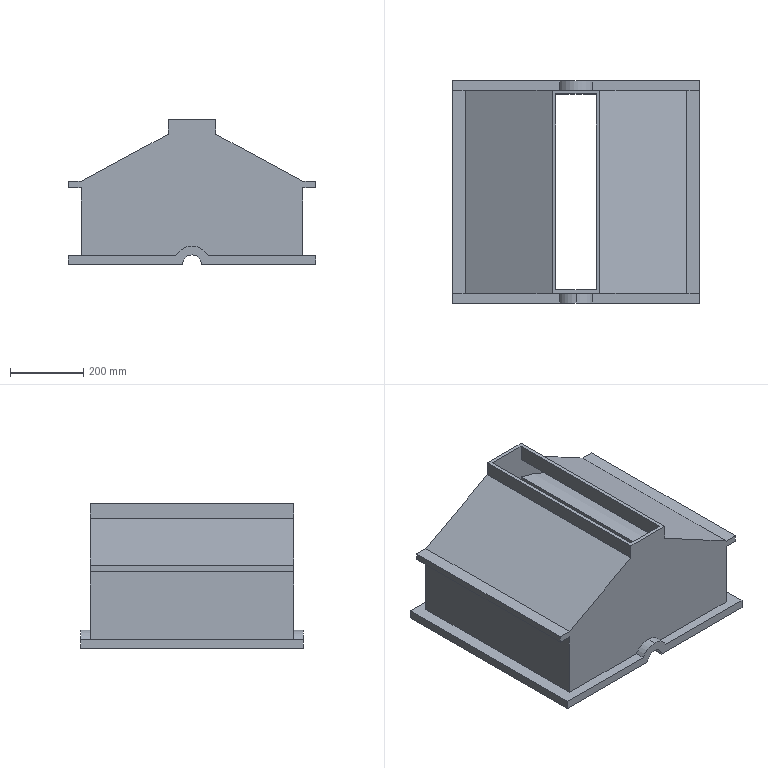Part | SolidWorks | features ICE 5, MirrorPattern 4, Extrusion 1 | 1 solid | 44 faces | box 677.491 x 608 x 396.469 mm | volume 20641288 mm3 | plane 33 | cylinder 11 | commonest cylinder face diameters 52 x4 100 x3 556 x2 596 x2
STEP:
#1=CARTESIAN_POINT('',(5.246,268.,26.));
#2=VERTEX_POINT('',#1);
#3=CARTESIAN_POINT('',(31.246,268.,0.));
#4=VERTEX_POINT('',#3);
#5=CARTESIAN_POINT('',(5.246,268.,0.));
#6=DIRECTION('',(0.,1.,0.));
#7=DIRECTION('',(0.,0.,1.));
#8=AXIS2_PLACEMENT_3D('',#5,#6,#7);
#9=CIRCLE('',#8,26.);
#10=EDGE_CURVE('',#2,#4,#9,.T.);
#11=ORIENTED_EDGE('',*,*,#10,.F.);
#12=CARTESIAN_POINT('',(5.246,304.,26.));
#13=VERTEX_POINT('',#12);
#14=CARTESIAN_POINT('',(5.246,-304.,26.));
#15=DIRECTION('',(0.,1.,0.));
#16=VECTOR('',#15,1000.);
#17=LINE('',#14,#16);
#18=EDGE_CURVE('',#2,#13,#17,.T.);
#19=ORIENTED_EDGE('',*,*,#18,.T.);
#20=CARTESIAN_POINT('',(31.246,304.,0.));
#21=VERTEX_POINT('',#20);
#22=CARTESIAN_POINT('',(5.246,304.,0.));
#23=DIRECTION('',(0.,1.,0.));
#24=DIRECTION('',(0.,0.,1.));
#25=AXIS2_PLACEMENT_3D('',#22,#23,#24);
#26=CIRCLE('',#25,26.);
#27=EDGE_CURVE('',#13,#21,#26,.T.);
#28=ORIENTED_EDGE('',*,*,#27,.T.);
#29=CARTESIAN_POINT('',(31.246,-304.,0.));
#30=DIRECTION('',(0.,1.,0.));
#31=VECTOR('',#30,1000.);
#32=LINE('',#29,#31);
#33=EDGE_CURVE('',#4,#21,#32,.T.);
#34=ORIENTED_EDGE('',*,*,#33,.F.);
#35=EDGE_LOOP('',(#11,#19,#28,#34));
#36=FACE_OUTER_BOUND('',#35,.T.);
#37=CARTESIAN_POINT('',(5.246,-304.,0.));
#38=DIRECTION('',(0.,1.,0.));
#39=DIRECTION('',(0.,0.,1.));
#40=AXIS2_PLACEMENT_3D('',#37,#38,#39);
#41=CYLINDRICAL_SURFACE('',#40,26.);
#42=ADVANCED_FACE('',(#36),#41,.F.);
#43=CARTESIAN_POINT('',(31.246,-304.,0.));
#44=VERTEX_POINT('',#43);
#45=CARTESIAN_POINT('',(5.246,-304.,26.));
#46=VERTEX_POINT('',#45);
#47=CARTESIAN_POINT('',(5.246,-304.,0.));
#48=DIRECTION('',(0.,-1.,0.));
#49=DIRECTION('',(0.,0.,-1.));
#50=AXIS2_PLACEMENT_3D('',#47,#48,#49);
#51=CIRCLE('',#50,26.);
#52=EDGE_CURVE('',#44,#46,#51,.T.);
#53=ORIENTED_EDGE('',*,*,#52,.T.);
#54=CARTESIAN_POINT('',(5.246,-268.,26.));
#55=VERTEX_POINT('',#54);
#56=CARTESIAN_POINT('',(5.246,-304.,26.));
#57=DIRECTION('',(0.,1.,0.));
#58=VECTOR('',#57,1000.);
#59=LINE('',#56,#58);
#60=EDGE_CURVE('',#46,#55,#59,.T.);
#61=ORIENTED_EDGE('',*,*,#60,.T.);
#62=CARTESIAN_POINT('',(31.246,-268.,0.));
#63=VERTEX_POINT('',#62);
#64=CARTESIAN_POINT('',(5.246,-268.,0.));
#65=DIRECTION('',(0.,-1.,0.));
#66=DIRECTION('',(0.,0.,-1.));
#67=AXIS2_PLACEMENT_3D('',#64,#65,#66);
#68=CIRCLE('',#67,26.);
#69=EDGE_CURVE('',#63,#55,#68,.T.);
#70=ORIENTED_EDGE('',*,*,#69,.F.);
#71=CARTESIAN_POINT('',(31.246,-304.,0.));
#72=DIRECTION('',(0.,1.,0.));
#73=VECTOR('',#72,1000.);
#74=LINE('',#71,#73);
#75=EDGE_CURVE('',#44,#63,#74,.T.);
#76=ORIENTED_EDGE('',*,*,#75,.F.);
#77=EDGE_LOOP('',(#53,#61,#70,#76));
#78=FACE_OUTER_BOUND('',#77,.T.);
#79=CARTESIAN_POINT('',(5.246,-304.,0.));
#80=DIRECTION('',(0.,1.,0.));
#81=DIRECTION('',(0.,0.,1.));
#82=AXIS2_PLACEMENT_3D('',#79,#80,#81);
#83=CYLINDRICAL_SURFACE('',#82,26.);
#84=ADVANCED_FACE('',(#78),#83,.F.);
#85=CARTESIAN_POINT('',(-38.618,-304.,24.));
#86=VERTEX_POINT('',#85);
#87=CARTESIAN_POINT('',(5.246,-304.,50.));
#88=VERTEX_POINT('',#87);
#89=CARTESIAN_POINT('',(5.246,-304.,0.));
#90=DIRECTION('',(0.,1.,0.));
#91=DIRECTION('',(0.,0.,1.));
#92=AXIS2_PLACEMENT_3D('',#89,#90,#91);
#93=CIRCLE('',#92,50.);
#94=EDGE_CURVE('',#86,#88,#93,.T.);
#95=ORIENTED_EDGE('',*,*,#94,.T.);
#96=CARTESIAN_POINT('',(5.246,-278.,50.));
#97=VERTEX_POINT('',#96);
#98=CARTESIAN_POINT('',(5.246,-304.,50.));
#99=DIRECTION('',(0.,1.,0.));
#100=VECTOR('',#99,1000.);
#101=LINE('',#98,#100);
#102=EDGE_CURVE('',#88,#97,#101,.T.);
#103=ORIENTED_EDGE('',*,*,#102,.T.);
#104=CARTESIAN_POINT('',(-38.618,-278.,24.));
#105=VERTEX_POINT('',#104);
#106=CARTESIAN_POINT('',(5.246,-278.,0.));
#107=DIRECTION('',(0.,1.,0.));
#108=DIRECTION('',(0.,0.,1.));
#109=AXIS2_PLACEMENT_3D('',#106,#107,#108);
#110=CIRCLE('',#109,50.);
#111=EDGE_CURVE('',#105,#97,#110,.T.);
#112=ORIENTED_EDGE('',*,*,#111,.F.);
#113=CARTESIAN_POINT('',(-38.618,-304.,24.));
#114=DIRECTION('',(0.,1.,0.));
#115=VECTOR('',#114,1000.);
#116=LINE('',#113,#115);
#117=EDGE_CURVE('',#86,#105,#116,.T.);
#118=ORIENTED_EDGE('',*,*,#117,.F.);
#119=EDGE_LOOP('',(#95,#103,#112,#118));
#120=FACE_OUTER_BOUND('',#119,.T.);
#121=CARTESIAN_POINT('',(5.246,-304.,0.));
#122=DIRECTION('',(0.,1.,0.));
#123=DIRECTION('',(0.,0.,1.));
#124=AXIS2_PLACEMENT_3D('',#121,#122,#123);
#125=CYLINDRICAL_SURFACE('',#124,50.);
#126=ADVANCED_FACE('',(#120),#125,.T.);
#127=CARTESIAN_POINT('',(343.991,-304.,0.));
#128=VERTEX_POINT('',#127);
#129=CARTESIAN_POINT('',(-333.5,-304.,0.));
#130=DIRECTION('',(1.,0.,0.));
#131=VECTOR('',#130,1000.);
#132=LINE('',#129,#131);
#133=EDGE_CURVE('',#44,#128,#132,.T.);
#134=ORIENTED_EDGE('',*,*,#133,.F.);
#135=ORIENTED_EDGE('',*,*,#75,.T.);
#136=CARTESIAN_POINT('',(288.491,-268.,0.));
#137=VERTEX_POINT('',#136);
#138=CARTESIAN_POINT('',(-298.,-268.,0.));
#139=DIRECTION('',(-1.,0.,0.));
#140=VECTOR('',#139,1000.);
#141=LINE('',#138,#140);
#142=EDGE_CURVE('',#137,#63,#141,.T.);
#143=ORIENTED_EDGE('',*,*,#142,.F.);
#144=CARTESIAN_POINT('',(288.491,268.,0.));
#145=VERTEX_POINT('',#144);
#146=CARTESIAN_POINT('',(288.491,278.,0.));
#147=DIRECTION('',(0.,-1.,0.));
#148=VECTOR('',#147,1000.);
#149=LINE('',#146,#148);
#150=EDGE_CURVE('',#145,#137,#149,.T.);
#151=ORIENTED_EDGE('',*,*,#150,.F.);
#152=CARTESIAN_POINT('',(-298.,268.,0.));
#153=DIRECTION('',(-1.,0.,0.));
#154=VECTOR('',#153,1000.);
#155=LINE('',#152,#154);
#156=EDGE_CURVE('',#145,#4,#155,.T.);
#157=ORIENTED_EDGE('',*,*,#156,.T.);
#158=ORIENTED_EDGE('',*,*,#33,.T.);
#159=CARTESIAN_POINT('',(343.991,304.,0.));
#160=VERTEX_POINT('',#159);
#161=CARTESIAN_POINT('',(-333.5,304.,0.));
#162=DIRECTION('',(1.,0.,0.));
#163=VECTOR('',#162,1000.);
#164=LINE('',#161,#163);
#165=EDGE_CURVE('',#21,#160,#164,.T.);
#166=ORIENTED_EDGE('',*,*,#165,.T.);
#167=CARTESIAN_POINT('',(343.991,278.,0.));
#168=DIRECTION('',(0.,-1.,0.));
#169=VECTOR('',#168,1000.);
#170=LINE('',#167,#169);
#171=EDGE_CURVE('',#160,#128,#170,.T.);
#172=ORIENTED_EDGE('',*,*,#171,.T.);
#173=EDGE_LOOP('',(#134,#135,#143,#151,#157,#158,#166,#172));
#174=FACE_OUTER_BOUND('',#173,.T.);
#175=CARTESIAN_POINT('',(0.,278.,0.));
#176=DIRECTION('',(0.,0.,1.));
#177=DIRECTION('',(1.,0.,0.));
#178=AXIS2_PLACEMENT_3D('',#175,#176,#177);
#179=PLANE('',#178);
#180=ADVANCED_FACE('',(#174),#179,.F.);
#181=CARTESIAN_POINT('',(308.491,-278.,24.));
#182=VERTEX_POINT('',#181);
#183=CARTESIAN_POINT('',(49.109,-278.,24.));
#184=VERTEX_POINT('',#183);
#185=CARTESIAN_POINT('',(343.991,-278.,24.));
#186=DIRECTION('',(-1.,0.,0.));
#187=VECTOR('',#186,1000.);
#188=LINE('',#185,#187);
#189=EDGE_CURVE('',#182,#184,#188,.T.);
#190=ORIENTED_EDGE('',*,*,#189,.F.);
#191=CARTESIAN_POINT('',(308.491,-278.,209.58));
#192=VERTEX_POINT('',#191);
#193=CARTESIAN_POINT('',(308.491,-278.,209.359));
#194=DIRECTION('',(0.,0.,1.));
#195=VECTOR('',#194,1000.);
#196=LINE('',#193,#195);
#197=EDGE_CURVE('',#182,#192,#196,.T.);
#198=ORIENTED_EDGE('',*,*,#197,.T.);
#199=CARTESIAN_POINT('',(343.991,-278.,209.58));
#200=VERTEX_POINT('',#199);
#201=CARTESIAN_POINT('',(10.491,-278.,209.58));
#202=DIRECTION('',(1.,0.,0.));
#203=VECTOR('',#202,1000.);
#204=LINE('',#201,#203);
#205=EDGE_CURVE('',#192,#200,#204,.T.);
#206=ORIENTED_EDGE('',*,*,#205,.T.);
#207=CARTESIAN_POINT('',(343.991,-278.,228.));
#208=VERTEX_POINT('',#207);
#209=CARTESIAN_POINT('',(343.991,-278.,0.));
#210=DIRECTION('',(0.,0.,1.));
#211=VECTOR('',#210,1000.);
#212=LINE('',#209,#211);
#213=EDGE_CURVE('',#200,#208,#212,.T.);
#214=ORIENTED_EDGE('',*,*,#213,.T.);
#215=CARTESIAN_POINT('',(308.491,-278.,228.));
#216=VERTEX_POINT('',#215);
#217=CARTESIAN_POINT('',(10.491,-278.,228.));
#218=DIRECTION('',(-1.,0.,0.));
#219=VECTOR('',#218,1000.);
#220=LINE('',#217,#219);
#221=EDGE_CURVE('',#208,#216,#220,.T.);
#222=ORIENTED_EDGE('',*,*,#221,.T.);
#223=CARTESIAN_POINT('',(70.491,-278.,356.469));
#224=VERTEX_POINT('',#223);
#225=CARTESIAN_POINT('',(308.491,-278.,228.));
#226=DIRECTION('',(-0.88,0.,0.475));
#227=VECTOR('',#226,1000.);
#228=LINE('',#225,#227);
#229=EDGE_CURVE('',#216,#224,#228,.T.);
#230=ORIENTED_EDGE('',*,*,#229,.T.);
#231=CARTESIAN_POINT('',(70.491,-278.,396.469));
#232=VERTEX_POINT('',#231);
#233=CARTESIAN_POINT('',(70.491,-278.,356.469));
#234=DIRECTION('',(0.,0.,1.));
#235=VECTOR('',#234,1000.);
#236=LINE('',#233,#235);
#237=EDGE_CURVE('',#224,#232,#236,.T.);
#238=ORIENTED_EDGE('',*,*,#237,.T.);
#239=CARTESIAN_POINT('',(-60.,-278.,396.469));
#240=VERTEX_POINT('',#239);
#241=CARTESIAN_POINT('',(0.,-278.,396.469));
#242=DIRECTION('',(-1.,0.,0.));
#243=VECTOR('',#242,1000.);
#244=LINE('',#241,#243);
#245=EDGE_CURVE('',#232,#240,#244,.T.);
#246=ORIENTED_EDGE('',*,*,#245,.T.);
#247=CARTESIAN_POINT('',(-60.,-278.,356.469));
#248=VERTEX_POINT('',#247);
#249=CARTESIAN_POINT('',(-60.,-278.,0.));
#250=DIRECTION('',(0.,0.,-1.));
#251=VECTOR('',#250,1000.);
#252=LINE('',#249,#251);
#253=EDGE_CURVE('',#240,#248,#252,.T.);
#254=ORIENTED_EDGE('',*,*,#253,.T.);
#255=CARTESIAN_POINT('',(-298.,-278.,228.));
#256=VERTEX_POINT('',#255);
#257=CARTESIAN_POINT('',(-162.54,-278.,301.119));
#258=DIRECTION('',(-0.88,0.,-0.475));
#259=VECTOR('',#258,1000.);
#260=LINE('',#257,#259);
#261=EDGE_CURVE('',#248,#256,#260,.T.);
#262=ORIENTED_EDGE('',*,*,#261,.T.);
#263=CARTESIAN_POINT('',(-333.5,-278.,228.));
#264=VERTEX_POINT('',#263);
#265=CARTESIAN_POINT('',(0.,-278.,228.));
#266=DIRECTION('',(1.,0.,0.));
#267=VECTOR('',#266,1000.);
#268=LINE('',#265,#267);
#269=EDGE_CURVE('',#264,#256,#268,.T.);
#270=ORIENTED_EDGE('',*,*,#269,.F.);
#271=CARTESIAN_POINT('',(-333.5,-278.,209.58));
#272=VERTEX_POINT('',#271);
#273=CARTESIAN_POINT('',(-333.5,-278.,0.));
#274=DIRECTION('',(0.,0.,1.));
#275=VECTOR('',#274,1000.);
#276=LINE('',#273,#275);
#277=EDGE_CURVE('',#272,#264,#276,.T.);
#278=ORIENTED_EDGE('',*,*,#277,.F.);
#279=CARTESIAN_POINT('',(-298.,-278.,209.58));
#280=VERTEX_POINT('',#279);
#281=CARTESIAN_POINT('',(0.,-278.,209.58));
#282=DIRECTION('',(-1.,0.,0.));
#283=VECTOR('',#282,1000.);
#284=LINE('',#281,#283);
#285=EDGE_CURVE('',#280,#272,#284,.T.);
#286=ORIENTED_EDGE('',*,*,#285,.F.);
#287=CARTESIAN_POINT('',(-298.,-278.,24.));
#288=VERTEX_POINT('',#287);
#289=CARTESIAN_POINT('',(-298.,-278.,0.));
#290=DIRECTION('',(0.,0.,1.));
#291=VECTOR('',#290,1000.);
#292=LINE('',#289,#291);
#293=EDGE_CURVE('',#288,#280,#292,.T.);
#294=ORIENTED_EDGE('',*,*,#293,.F.);
#295=CARTESIAN_POINT('',(-333.5,-278.,24.));
#296=DIRECTION('',(1.,0.,0.));
#297=VECTOR('',#296,1000.);
#298=LINE('',#295,#297);
#299=EDGE_CURVE('',#288,#105,#298,.T.);
#300=ORIENTED_EDGE('',*,*,#299,.T.);
#301=ORIENTED_EDGE('',*,*,#111,.T.);
#302=CARTESIAN_POINT('',(5.246,-278.,0.));
#303=DIRECTION('',(0.,1.,0.));
#304=DIRECTION('',(0.,0.,1.));
#305=AXIS2_PLACEMENT_3D('',#302,#303,#304);
#306=CIRCLE('',#305,50.);
#307=EDGE_CURVE('',#97,#184,#306,.T.);
#308=ORIENTED_EDGE('',*,*,#307,.T.);
#309=EDGE_LOOP('',(#190,#198,#206,#214,#222,#230,#238,#246,#254,#262,#270,#278,#286,#294,#300,#301,#308));
#310=FACE_OUTER_BOUND('',#309,.T.);
#311=CARTESIAN_POINT('',(0.,-278.,0.));
#312=DIRECTION('',(0.,1.,0.));
#313=DIRECTION('',(0.,0.,1.));
#314=AXIS2_PLACEMENT_3D('',#311,#312,#313);
#315=PLANE('',#314);
#316=ADVANCED_FACE('',(#310),#315,.F.);
#317=CARTESIAN_POINT('',(49.109,278.,24.));
#318=VERTEX_POINT('',#317);
#319=CARTESIAN_POINT('',(308.491,278.,24.));
#320=VERTEX_POINT('',#319);
#321=CARTESIAN_POINT('',(343.991,278.,24.));
#322=DIRECTION('',(1.,0.,0.));
#323=VECTOR('',#322,1000.);
#324=LINE('',#321,#323);
#325=EDGE_CURVE('',#318,#320,#324,.T.);
#326=ORIENTED_EDGE('',*,*,#325,.F.);
#327=CARTESIAN_POINT('',(-38.618,278.,24.));
#328=VERTEX_POINT('',#327);
#329=CARTESIAN_POINT('',(5.246,278.,0.));
#330=DIRECTION('',(0.,1.,0.));
#331=DIRECTION('',(0.,0.,1.));
#332=AXIS2_PLACEMENT_3D('',#329,#330,#331);
#333=CIRCLE('',#332,50.);
#334=EDGE_CURVE('',#328,#318,#333,.T.);
#335=ORIENTED_EDGE('',*,*,#334,.F.);
#336=CARTESIAN_POINT('',(-298.,278.,24.));
#337=VERTEX_POINT('',#336);
#338=CARTESIAN_POINT('',(-333.5,278.,24.));
#339=DIRECTION('',(1.,0.,0.));
#340=VECTOR('',#339,1000.);
#341=LINE('',#338,#340);
#342=EDGE_CURVE('',#337,#328,#341,.T.);
#343=ORIENTED_EDGE('',*,*,#342,.F.);
#344=CARTESIAN_POINT('',(-298.,278.,209.58));
#345=VERTEX_POINT('',#344);
#346=CARTESIAN_POINT('',(-298.,278.,0.));
#347=DIRECTION('',(0.,0.,1.));
#348=VECTOR('',#347,1000.);
#349=LINE('',#346,#348);
#350=EDGE_CURVE('',#337,#345,#349,.T.);
#351=ORIENTED_EDGE('',*,*,#350,.T.);
#352=CARTESIAN_POINT('',(-333.5,278.,209.58));
#353=VERTEX_POINT('',#352);
#354=CARTESIAN_POINT('',(0.,278.,209.58));
#355=DIRECTION('',(-1.,0.,0.));
#356=VECTOR('',#355,1000.);
#357=LINE('',#354,#356);
#358=EDGE_CURVE('',#345,#353,#357,.T.);
#359=ORIENTED_EDGE('',*,*,#358,.T.);
#360=CARTESIAN_POINT('',(-333.5,278.,228.));
#361=VERTEX_POINT('',#360);
#362=CARTESIAN_POINT('',(-333.5,278.,0.));
#363=DIRECTION('',(0.,0.,1.));
#364=VECTOR('',#363,1000.);
#365=LINE('',#362,#364);
#366=EDGE_CURVE('',#353,#361,#365,.T.);
#367=ORIENTED_EDGE('',*,*,#366,.T.);
#368=CARTESIAN_POINT('',(-298.,278.,228.));
#369=VERTEX_POINT('',#368);
#370=CARTESIAN_POINT('',(0.,278.,228.));
#371=DIRECTION('',(1.,0.,0.));
#372=VECTOR('',#371,1000.);
#373=LINE('',#370,#372);
#374=EDGE_CURVE('',#361,#369,#373,.T.);
#375=ORIENTED_EDGE('',*,*,#374,.T.);
#376=CARTESIAN_POINT('',(-60.,278.,356.469));
#377=VERTEX_POINT('',#376);
#378=CARTESIAN_POINT('',(-162.54,278.,301.119));
#379=DIRECTION('',(-0.88,0.,-0.475));
#380=VECTOR('',#379,1000.);
#381=LINE('',#378,#380);
#382=EDGE_CURVE('',#377,#369,#381,.T.);
#383=ORIENTED_EDGE('',*,*,#382,.F.);
#384=CARTESIAN_POINT('',(-60.,278.,396.469));
#385=VERTEX_POINT('',#384);
#386=CARTESIAN_POINT('',(-60.,278.,0.));
#387=DIRECTION('',(0.,0.,-1.));
#388=VECTOR('',#387,1000.);
#389=LINE('',#386,#388);
#390=EDGE_CURVE('',#385,#377,#389,.T.);
#391=ORIENTED_EDGE('',*,*,#390,.F.);
#392=CARTESIAN_POINT('',(70.491,278.,396.469));
#393=VERTEX_POINT('',#392);
#394=CARTESIAN_POINT('',(0.,278.,396.469));
#395=DIRECTION('',(-1.,0.,0.));
#396=VECTOR('',#395,1000.);
#397=LINE('',#394,#396);
#398=EDGE_CURVE('',#393,#385,#397,.T.);
#399=ORIENTED_EDGE('',*,*,#398,.F.);
#400=CARTESIAN_POINT('',(70.491,278.,356.469));
#401=VERTEX_POINT('',#400);
#402=CARTESIAN_POINT('',(70.491,278.,356.469));
#403=DIRECTION('',(0.,0.,1.));
#404=VECTOR('',#403,1000.);
#405=LINE('',#402,#404);
#406=EDGE_CURVE('',#401,#393,#405,.T.);
#407=ORIENTED_EDGE('',*,*,#406,.F.);
#408=CARTESIAN_POINT('',(308.491,278.,228.));
#409=VERTEX_POINT('',#408);
#410=CARTESIAN_POINT('',(308.491,278.,228.));
#411=DIRECTION('',(-0.88,0.,0.475));
#412=VECTOR('',#411,1000.);
#413=LINE('',#410,#412);
#414=EDGE_CURVE('',#409,#401,#413,.T.);
#415=ORIENTED_EDGE('',*,*,#414,.F.);
#416=CARTESIAN_POINT('',(343.991,278.,228.));
#417=VERTEX_POINT('',#416);
#418=CARTESIAN_POINT('',(10.491,278.,228.));
#419=DIRECTION('',(-1.,0.,0.));
#420=VECTOR('',#419,1000.);
#421=LINE('',#418,#420);
#422=EDGE_CURVE('',#417,#409,#421,.T.);
#423=ORIENTED_EDGE('',*,*,#422,.F.);
#424=CARTESIAN_POINT('',(343.991,278.,209.58));
#425=VERTEX_POINT('',#424);
#426=CARTESIAN_POINT('',(343.991,278.,0.));
#427=DIRECTION('',(0.,0.,1.));
#428=VECTOR('',#427,1000.);
#429=LINE('',#426,#428);
#430=EDGE_CURVE('',#425,#417,#429,.T.);
#431=ORIENTED_EDGE('',*,*,#430,.F.);
#432=CARTESIAN_POINT('',(308.491,278.,209.58));
#433=VERTEX_POINT('',#432);
#434=CARTESIAN_POINT('',(10.491,278.,209.58));
#435=DIRECTION('',(1.,0.,0.));
#436=VECTOR('',#435,1000.);
#437=LINE('',#434,#436);
#438=EDGE_CURVE('',#433,#425,#437,.T.);
#439=ORIENTED_EDGE('',*,*,#438,.F.);
#440=CARTESIAN_POINT('',(308.491,278.,209.359));
#441=DIRECTION('',(0.,0.,1.));
#442=VECTOR('',#441,1000.);
#443=LINE('',#440,#442);
#444=EDGE_CURVE('',#320,#433,#443,.T.);
#445=ORIENTED_EDGE('',*,*,#444,.F.);
#446=EDGE_LOOP('',(#326,#335,#343,#351,#359,#367,#375,#383,#391,#399,#407,#415,#423,#431,#439,#445));
#447=FACE_OUTER_BOUND('',#446,.T.);
#448=CARTESIAN_POINT('',(0.,278.,0.));
#449=DIRECTION('',(0.,1.,0.));
#450=DIRECTION('',(0.,0.,1.));
#451=AXIS2_PLACEMENT_3D('',#448,#449,#450);
#452=PLANE('',#451);
#453=ADVANCED_FACE('',(#447),#452,.T.);
#454=CARTESIAN_POINT('',(-286.793,-268.,80.955));
#455=VERTEX_POINT('',#454);
#456=CARTESIAN_POINT('',(-285.175,-268.,220.714));
#457=VERTEX_POINT('',#456);
#458=CARTESIAN_POINT('',(-287.692,-268.,3.331));
#459=DIRECTION('',(0.01158,0.,0.9999));
#460=VECTOR('',#459,1000.);
#461=LINE('',#458,#460);
#462=EDGE_CURVE('',#455,#457,#461,.T.);
#463=ORIENTED_EDGE('',*,*,#462,.F.);
#464=CARTESIAN_POINT('',(-286.793,268.,80.955));
#465=VERTEX_POINT('',#464);
#466=CARTESIAN_POINT('',(-286.793,278.,80.955));
#467=DIRECTION('',(0.,-1.,0.));
#468=VECTOR('',#467,1000.);
#469=LINE('',#466,#468);
#470=EDGE_CURVE('',#465,#455,#469,.T.);
#471=ORIENTED_EDGE('',*,*,#470,.F.);
#472=CARTESIAN_POINT('',(-285.175,268.,220.714));
#473=VERTEX_POINT('',#472);
#474=CARTESIAN_POINT('',(-287.692,268.,3.331));
#475=DIRECTION('',(-0.01158,0.,-0.9999));
#476=VECTOR('',#475,1000.);
#477=LINE('',#474,#476);
#478=EDGE_CURVE('',#473,#465,#477,.T.);
#479=ORIENTED_EDGE('',*,*,#478,.F.);
#480=CARTESIAN_POINT('',(-285.175,278.,220.714));
#481=DIRECTION('',(0.,-1.,0.));
#482=VECTOR('',#481,1000.);
#483=LINE('',#480,#482);
#484=EDGE_CURVE('',#473,#457,#483,.T.);
#485=ORIENTED_EDGE('',*,*,#484,.T.);
#486=EDGE_LOOP('',(#463,#471,#479,#485));
#487=FACE_OUTER_BOUND('',#486,.T.);
#488=CARTESIAN_POINT('',(-287.692,278.,3.331));
#489=DIRECTION('',(-0.9999,0.,0.01158));
#490=DIRECTION('',(0.01158,0.,0.9999));
#491=AXIS2_PLACEMENT_3D('',#488,#489,#490);
#492=PLANE('',#491);
#493=ADVANCED_FACE('',(#487),#492,.F.);
#494=CARTESIAN_POINT('',(-49.909,-268.,293.791));
#495=VERTEX_POINT('',#494);
#496=CARTESIAN_POINT('',(0.,-268.,0.));
#497=DIRECTION('',(0.,-1.,0.));
#498=DIRECTION('',(0.,0.,-1.));
#499=AXIS2_PLACEMENT_3D('',#496,#497,#498);
#500=CIRCLE('',#499,298.);
#501=EDGE_CURVE('',#495,#455,#500,.T.);
#502=ORIENTED_EDGE('',*,*,#501,.F.);
#503=CARTESIAN_POINT('',(-49.909,268.,293.791));
#504=VERTEX_POINT('',#503);
#505=CARTESIAN_POINT('',(-49.909,278.,293.791));
#506=DIRECTION('',(0.,-1.,0.));
#507=VECTOR('',#506,1000.);
#508=LINE('',#505,#507);
#509=EDGE_CURVE('',#504,#495,#508,.T.);
#510=ORIENTED_EDGE('',*,*,#509,.F.);
#511=CARTESIAN_POINT('',(0.,268.,0.));
#512=DIRECTION('',(0.,1.,0.));
#513=DIRECTION('',(0.,0.,1.));
#514=AXIS2_PLACEMENT_3D('',#511,#512,#513);
#515=CIRCLE('',#514,298.);
#516=EDGE_CURVE('',#465,#504,#515,.T.);
#517=ORIENTED_EDGE('',*,*,#516,.F.);
#518=ORIENTED_EDGE('',*,*,#470,.T.);
#519=EDGE_LOOP('',(#502,#510,#517,#518));
#520=FACE_OUTER_BOUND('',#519,.T.);
#521=CARTESIAN_POINT('',(0.,278.,0.));
#522=DIRECTION('',(0.,-1.,0.));
#523=DIRECTION('',(0.,0.,-1.));
#524=AXIS2_PLACEMENT_3D('',#521,#522,#523);
#525=CYLINDRICAL_SURFACE('',#524,298.);
#526=ADVANCED_FACE('',(#520),#525,.T.);
#527=ORIENTED_EDGE('',*,*,#509,.T.);
#528=CARTESIAN_POINT('',(-49.909,-268.,273.483));
#529=VERTEX_POINT('',#528);
#530=CARTESIAN_POINT('',(-49.909,-268.,0.));
#531=DIRECTION('',(0.,0.,-1.));
#532=VECTOR('',#531,1000.);
#533=LINE('',#530,#532);
#534=EDGE_CURVE('',#495,#529,#533,.T.);
#535=ORIENTED_EDGE('',*,*,#534,.T.);
#536=CARTESIAN_POINT('',(-49.909,268.,273.483));
#537=VERTEX_POINT('',#536);
#538=CARTESIAN_POINT('',(-49.909,278.,273.483));
#539=DIRECTION('',(0.,-1.,0.));
#540=VECTOR('',#539,1000.);
#541=LINE('',#538,#540);
#542=EDGE_CURVE('',#537,#529,#541,.T.);
#543=ORIENTED_EDGE('',*,*,#542,.F.);
#544=CARTESIAN_POINT('',(-49.909,268.,0.));
#545=DIRECTION('',(0.,0.,1.));
#546=VECTOR('',#545,1000.);
#547=LINE('',#544,#546);
#548=EDGE_CURVE('',#537,#504,#547,.T.);
#549=ORIENTED_EDGE('',*,*,#548,.T.);
#550=EDGE_LOOP('',(#527,#535,#543,#549));
#551=FACE_OUTER_BOUND('',#550,.T.);
#552=CARTESIAN_POINT('',(-49.909,278.,0.));
#553=DIRECTION('',(1.,0.,0.));
#554=DIRECTION('',(0.,0.,-1.));
#555=AXIS2_PLACEMENT_3D('',#552,#553,#554);
#556=PLANE('',#555);
#557=ADVANCED_FACE('',(#551),#556,.T.);
#558=ORIENTED_EDGE('',*,*,#542,.T.);
#559=CARTESIAN_POINT('',(-278.,-268.,0.));
#560=VERTEX_POINT('',#559);
#561=CARTESIAN_POINT('',(0.,-268.,0.));
#562=DIRECTION('',(0.,-1.,0.));
#563=DIRECTION('',(0.,0.,-1.));
#564=AXIS2_PLACEMENT_3D('',#561,#562,#563);
#565=CIRCLE('',#564,278.);
#566=EDGE_CURVE('',#529,#560,#565,.T.);
#567=ORIENTED_EDGE('',*,*,#566,.T.);
#568=CARTESIAN_POINT('',(-278.,268.,0.));
#569=VERTEX_POINT('',#568);
#570=CARTESIAN_POINT('',(-278.,278.,0.));
#571=DIRECTION('',(0.,-1.,0.));
#572=VECTOR('',#571,1000.);
#573=LINE('',#570,#572);
#574=EDGE_CURVE('',#569,#560,#573,.T.);
#575=ORIENTED_EDGE('',*,*,#574,.F.);
#576=CARTESIAN_POINT('',(0.,268.,0.));
#577=DIRECTION('',(0.,1.,0.));
#578=DIRECTION('',(0.,0.,1.));
#579=AXIS2_PLACEMENT_3D('',#576,#577,#578);
#580=CIRCLE('',#579,278.);
#581=EDGE_CURVE('',#569,#537,#580,.T.);
#582=ORIENTED_EDGE('',*,*,#581,.T.);
#583=EDGE_LOOP('',(#558,#567,#575,#582));
#584=FACE_OUTER_BOUND('',#583,.T.);
#585=CARTESIAN_POINT('',(0.,278.,0.));
#586=DIRECTION('',(0.,-1.,0.));
#587=DIRECTION('',(0.,0.,-1.));
#588=AXIS2_PLACEMENT_3D('',#585,#586,#587);
#589=CYLINDRICAL_SURFACE('',#588,278.);
#590=ADVANCED_FACE('',(#584),#589,.F.);
#591=CARTESIAN_POINT('',(-49.909,-268.,352.336));
#592=VERTEX_POINT('',#591);
#593=CARTESIAN_POINT('',(-49.909,-268.,396.469));
#594=VERTEX_POINT('',#593);
#595=CARTESIAN_POINT('',(-49.909,-268.,0.));
#596=DIRECTION('',(0.,0.,1.));
#597=VECTOR('',#596,1000.);
#598=LINE('',#595,#597);
#599=EDGE_CURVE('',#592,#594,#598,.T.);
#600=ORIENTED_EDGE('',*,*,#599,.F.);
#601=CARTESIAN_POINT('',(-49.909,268.,352.336));
#602=VERTEX_POINT('',#601);
#603=CARTESIAN_POINT('',(-49.909,278.,352.336));
#604=DIRECTION('',(0.,-1.,0.));
#605=VECTOR('',#604,1000.);
#606=LINE('',#603,#605);
#607=EDGE_CURVE('',#602,#592,#606,.T.);
#608=ORIENTED_EDGE('',*,*,#607,.F.);
#609=CARTESIAN_POINT('',(-49.909,268.,396.469));
#610=VERTEX_POINT('',#609);
#611=CARTESIAN_POINT('',(-49.909,268.,0.));
#612=DIRECTION('',(0.,0.,-1.));
#613=VECTOR('',#612,1000.);
#614=LINE('',#611,#613);
#615=EDGE_CURVE('',#610,#602,#614,.T.);
#616=ORIENTED_EDGE('',*,*,#615,.F.);
#617=CARTESIAN_POINT('',(-49.909,278.,396.469));
#618=DIRECTION('',(0.,-1.,0.));
#619=VECTOR('',#618,1000.);
#620=LINE('',#617,#619);
#621=EDGE_CURVE('',#610,#594,#620,.T.);
#622=ORIENTED_EDGE('',*,*,#621,.T.);
#623=EDGE_LOOP('',(#600,#608,#616,#622));
#624=FACE_OUTER_BOUND('',#623,.T.);
#625=CARTESIAN_POINT('',(-49.909,278.,0.));
#626=DIRECTION('',(-1.,0.,0.));
#627=DIRECTION('',(0.,0.,1.));
#628=AXIS2_PLACEMENT_3D('',#625,#626,#627);
#629=PLANE('',#628);
#630=ADVANCED_FACE('',(#624),#629,.F.);
#631=CARTESIAN_POINT('',(-162.026,-268.,289.611));
#632=DIRECTION('',(0.8727,0.,0.4882));
#633=VECTOR('',#632,1000.);
#634=LINE('',#631,#633);
#635=EDGE_CURVE('',#457,#592,#634,.T.);
#636=ORIENTED_EDGE('',*,*,#635,.F.);
#637=ORIENTED_EDGE('',*,*,#484,.F.);
#638=CARTESIAN_POINT('',(-162.026,268.,289.611));
#639=DIRECTION('',(-0.8727,0.,-0.4882));
#640=VECTOR('',#639,1000.);
#641=LINE('',#638,#640);
#642=EDGE_CURVE('',#602,#473,#641,.T.);
#643=ORIENTED_EDGE('',*,*,#642,.F.);
#644=ORIENTED_EDGE('',*,*,#607,.T.);
#645=EDGE_LOOP('',(#636,#637,#643,#644));
#646=FACE_OUTER_BOUND('',#645,.T.);
#647=CARTESIAN_POINT('',(-162.026,278.,289.611));
#648=DIRECTION('',(-0.4882,0.,0.8727));
#649=DIRECTION('',(0.8727,0.,0.4882));
#650=AXIS2_PLACEMENT_3D('',#647,#648,#649);
#651=PLANE('',#650);
#652=ADVANCED_FACE('',(#646),#651,.F.);
#653=CARTESIAN_POINT('',(-333.5,304.,0.));
#654=VERTEX_POINT('',#653);
#655=CARTESIAN_POINT('',(-20.754,304.,0.));
#656=VERTEX_POINT('',#655);
#657=CARTESIAN_POINT('',(-333.5,304.,0.));
#658=DIRECTION('',(1.,0.,0.));
#659=VECTOR('',#658,1000.);
#660=LINE('',#657,#659);
#661=EDGE_CURVE('',#654,#656,#660,.T.);
#662=ORIENTED_EDGE('',*,*,#661,.T.);
#663=CARTESIAN_POINT('',(-20.754,268.,0.));
#664=VERTEX_POINT('',#663);
#665=CARTESIAN_POINT('',(-20.754,-304.,0.));
#666=DIRECTION('',(0.,-1.,0.));
#667=VECTOR('',#666,1000.);
#668=LINE('',#665,#667);
#669=EDGE_CURVE('',#656,#664,#668,.T.);
#670=ORIENTED_EDGE('',*,*,#669,.T.);
#671=CARTESIAN_POINT('',(-298.,268.,0.));
#672=DIRECTION('',(-1.,0.,0.));
#673=VECTOR('',#672,1000.);
#674=LINE('',#671,#673);
#675=EDGE_CURVE('',#664,#569,#674,.T.);
#676=ORIENTED_EDGE('',*,*,#675,.T.);
#677=ORIENTED_EDGE('',*,*,#574,.T.);
#678=CARTESIAN_POINT('',(-20.754,-268.,0.));
#679=VERTEX_POINT('',#678);
#680=CARTESIAN_POINT('',(-298.,-268.,0.));
#681=DIRECTION('',(-1.,0.,0.));
#682=VECTOR('',#681,1000.);
#683=LINE('',#680,#682);
#684=EDGE_CURVE('',#679,#560,#683,.T.);
#685=ORIENTED_EDGE('',*,*,#684,.F.);
#686=CARTESIAN_POINT('',(-20.754,-304.,0.));
#687=VERTEX_POINT('',#686);
#688=CARTESIAN_POINT('',(-20.754,-304.,0.));
#689=DIRECTION('',(0.,-1.,0.));
#690=VECTOR('',#689,1000.);
#691=LINE('',#688,#690);
#692=EDGE_CURVE('',#679,#687,#691,.T.);
#693=ORIENTED_EDGE('',*,*,#692,.T.);
#694=CARTESIAN_POINT('',(-333.5,-304.,0.));
#695=VERTEX_POINT('',#694);
#696=CARTESIAN_POINT('',(-333.5,-304.,0.));
#697=DIRECTION('',(1.,0.,0.));
#698=VECTOR('',#697,1000.);
#699=LINE('',#696,#698);
#700=EDGE_CURVE('',#695,#687,#699,.T.);
#701=ORIENTED_EDGE('',*,*,#700,.F.);
#702=CARTESIAN_POINT('',(-333.5,278.,0.));
#703=DIRECTION('',(0.,-1.,0.));
#704=VECTOR('',#703,1000.);
#705=LINE('',#702,#704);
#706=EDGE_CURVE('',#654,#695,#705,.T.);
#707=ORIENTED_EDGE('',*,*,#706,.F.);
#708=EDGE_LOOP('',(#662,#670,#676,#677,#685,#693,#701,#707));
#709=FACE_OUTER_BOUND('',#708,.T.);
#710=CARTESIAN_POINT('',(0.,278.,0.));
#711=DIRECTION('',(0.,0.,1.));
#712=DIRECTION('',(1.,0.,0.));
#713=AXIS2_PLACEMENT_3D('',#710,#711,#712);
#714=PLANE('',#713);
#715=ADVANCED_FACE('',(#709),#714,.F.);
#716=ORIENTED_EDGE('',*,*,#706,.T.);
#717=CARTESIAN_POINT('',(-333.5,-304.,24.));
#718=VERTEX_POINT('',#717);
#719=CARTESIAN_POINT('',(-333.5,-304.,24.));
#720=DIRECTION('',(0.,0.,-1.));
#721=VECTOR('',#720,1000.);
#722=LINE('',#719,#721);
#723=EDGE_CURVE('',#718,#695,#722,.T.);
#724=ORIENTED_EDGE('',*,*,#723,.F.);
#725=CARTESIAN_POINT('',(-333.5,304.,24.));
#726=VERTEX_POINT('',#725);
#727=CARTESIAN_POINT('',(-333.5,278.,24.));
#728=DIRECTION('',(0.,-1.,0.));
#729=VECTOR('',#728,1000.);
#730=LINE('',#727,#729);
#731=EDGE_CURVE('',#726,#718,#730,.T.);
#732=ORIENTED_EDGE('',*,*,#731,.F.);
#733=CARTESIAN_POINT('',(-333.5,304.,24.));
#734=DIRECTION('',(0.,0.,-1.));
#735=VECTOR('',#734,1000.);
#736=LINE('',#733,#735);
#737=EDGE_CURVE('',#726,#654,#736,.T.);
#738=ORIENTED_EDGE('',*,*,#737,.T.);
#739=EDGE_LOOP('',(#716,#724,#732,#738));
#740=FACE_OUTER_BOUND('',#739,.T.);
#741=CARTESIAN_POINT('',(-333.5,278.,0.));
#742=DIRECTION('',(1.,0.,0.));
#743=DIRECTION('',(0.,0.,-1.));
#744=AXIS2_PLACEMENT_3D('',#741,#742,#743);
#745=PLANE('',#744);
#746=ADVANCED_FACE('',(#740),#745,.F.);
#747=ORIENTED_EDGE('',*,*,#731,.T.);
#748=CARTESIAN_POINT('',(-333.5,-304.,24.));
#749=DIRECTION('',(1.,0.,0.));
#750=VECTOR('',#749,1000.);
#751=LINE('',#748,#750);
#752=EDGE_CURVE('',#718,#86,#751,.T.);
#753=ORIENTED_EDGE('',*,*,#752,.T.);
#754=ORIENTED_EDGE('',*,*,#117,.T.);
#755=ORIENTED_EDGE('',*,*,#299,.F.);
#756=CARTESIAN_POINT('',(-298.,278.,24.));
#757=DIRECTION('',(0.,-1.,0.));
#758=VECTOR('',#757,1000.);
#759=LINE('',#756,#758);
#760=EDGE_CURVE('',#337,#288,#759,.T.);
#761=ORIENTED_EDGE('',*,*,#760,.F.);
#762=ORIENTED_EDGE('',*,*,#342,.T.);
#763=CARTESIAN_POINT('',(-38.618,304.,24.));
#764=VERTEX_POINT('',#763);
#765=CARTESIAN_POINT('',(-38.618,304.,24.));
#766=DIRECTION('',(0.,-1.,0.));
#767=VECTOR('',#766,1000.);
#768=LINE('',#765,#767);
#769=EDGE_CURVE('',#764,#328,#768,.T.);
#770=ORIENTED_EDGE('',*,*,#769,.F.);
#771=CARTESIAN_POINT('',(-333.5,304.,24.));
#772=DIRECTION('',(1.,0.,0.));
#773=VECTOR('',#772,1000.);
#774=LINE('',#771,#773);
#775=EDGE_CURVE('',#726,#764,#774,.T.);
#776=ORIENTED_EDGE('',*,*,#775,.F.);
#777=EDGE_LOOP('',(#747,#753,#754,#755,#761,#762,#770,#776));
#778=FACE_OUTER_BOUND('',#777,.T.);
#779=CARTESIAN_POINT('',(0.,278.,24.));
#780=DIRECTION('',(0.,0.,-1.));
#781=DIRECTION('',(-1.,0.,0.));
#782=AXIS2_PLACEMENT_3D('',#779,#780,#781);
#783=PLANE('',#782);
#784=ADVANCED_FACE('',(#778),#783,.F.);
#785=ORIENTED_EDGE('',*,*,#293,.T.);
#786=CARTESIAN_POINT('',(-298.,278.,209.58));
#787=DIRECTION('',(0.,-1.,0.));
#788=VECTOR('',#787,1000.);
#789=LINE('',#786,#788);
#790=EDGE_CURVE('',#345,#280,#789,.T.);
#791=ORIENTED_EDGE('',*,*,#790,.F.);
#792=ORIENTED_EDGE('',*,*,#350,.F.);
#793=ORIENTED_EDGE('',*,*,#760,.T.);
#794=EDGE_LOOP('',(#785,#791,#792,#793));
#795=FACE_OUTER_BOUND('',#794,.T.);
#796=CARTESIAN_POINT('',(-298.,278.,0.));
#797=DIRECTION('',(1.,0.,0.));
#798=DIRECTION('',(0.,0.,-1.));
#799=AXIS2_PLACEMENT_3D('',#796,#797,#798);
#800=PLANE('',#799);
#801=ADVANCED_FACE('',(#795),#800,.F.);
#802=ORIENTED_EDGE('',*,*,#285,.T.);
#803=CARTESIAN_POINT('',(-333.5,278.,209.58));
#804=DIRECTION('',(0.,-1.,0.));
#805=VECTOR('',#804,1000.);
#806=LINE('',#803,#805);
#807=EDGE_CURVE('',#353,#272,#806,.T.);
#808=ORIENTED_EDGE('',*,*,#807,.F.);
#809=ORIENTED_EDGE('',*,*,#358,.F.);
#810=ORIENTED_EDGE('',*,*,#790,.T.);
#811=EDGE_LOOP('',(#802,#808,#809,#810));
#812=FACE_OUTER_BOUND('',#811,.T.);
#813=CARTESIAN_POINT('',(0.,278.,209.58));
#814=DIRECTION('',(0.,0.,1.));
#815=DIRECTION('',(1.,0.,0.));
#816=AXIS2_PLACEMENT_3D('',#813,#814,#815);
#817=PLANE('',#816);
#818=ADVANCED_FACE('',(#812),#817,.F.);
#819=ORIENTED_EDGE('',*,*,#277,.T.);
#820=CARTESIAN_POINT('',(-333.5,278.,228.));
#821=DIRECTION('',(0.,-1.,0.));
#822=VECTOR('',#821,1000.);
#823=LINE('',#820,#822);
#824=EDGE_CURVE('',#361,#264,#823,.T.);
#825=ORIENTED_EDGE('',*,*,#824,.F.);
#826=ORIENTED_EDGE('',*,*,#366,.F.);
#827=ORIENTED_EDGE('',*,*,#807,.T.);
#828=EDGE_LOOP('',(#819,#825,#826,#827));
#829=FACE_OUTER_BOUND('',#828,.T.);
#830=CARTESIAN_POINT('',(-333.5,278.,0.));
#831=DIRECTION('',(1.,0.,0.));
#832=DIRECTION('',(0.,0.,-1.));
#833=AXIS2_PLACEMENT_3D('',#830,#831,#832);
#834=PLANE('',#833);
#835=ADVANCED_FACE('',(#829),#834,.F.);
#836=ORIENTED_EDGE('',*,*,#269,.T.);
#837=CARTESIAN_POINT('',(-298.,278.,228.));
#838=DIRECTION('',(0.,-1.,0.));
#839=VECTOR('',#838,1000.);
#840=LINE('',#837,#839);
#841=EDGE_CURVE('',#369,#256,#840,.T.);
#842=ORIENTED_EDGE('',*,*,#841,.F.);
#843=ORIENTED_EDGE('',*,*,#374,.F.);
#844=ORIENTED_EDGE('',*,*,#824,.T.);
#845=EDGE_LOOP('',(#836,#842,#843,#844));
#846=FACE_OUTER_BOUND('',#845,.T.);
#847=CARTESIAN_POINT('',(0.,278.,228.));
#848=DIRECTION('',(0.,0.,-1.));
#849=DIRECTION('',(-1.,0.,0.));
#850=AXIS2_PLACEMENT_3D('',#847,#848,#849);
#851=PLANE('',#850);
#852=ADVANCED_FACE('',(#846),#851,.F.);
#853=ORIENTED_EDGE('',*,*,#261,.F.);
#854=CARTESIAN_POINT('',(-60.,278.,356.469));
#855=DIRECTION('',(0.,-1.,0.));
#856=VECTOR('',#855,1000.);
#857=LINE('',#854,#856);
#858=EDGE_CURVE('',#377,#248,#857,.T.);
#859=ORIENTED_EDGE('',*,*,#858,.F.);
#860=ORIENTED_EDGE('',*,*,#382,.T.);
#861=ORIENTED_EDGE('',*,*,#841,.T.);
#862=EDGE_LOOP('',(#853,#859,#860,#861));
#863=FACE_OUTER_BOUND('',#862,.T.);
#864=CARTESIAN_POINT('',(-162.54,278.,301.119));
#865=DIRECTION('',(-0.475,0.,0.88));
#866=DIRECTION('',(0.88,0.,0.475));
#867=AXIS2_PLACEMENT_3D('',#864,#865,#866);
#868=PLANE('',#867);
#869=ADVANCED_FACE('',(#863),#868,.T.);
#870=ORIENTED_EDGE('',*,*,#253,.F.);
#871=CARTESIAN_POINT('',(-60.,278.,396.469));
#872=DIRECTION('',(0.,-1.,0.));
#873=VECTOR('',#872,1000.);
#874=LINE('',#871,#873);
#875=EDGE_CURVE('',#385,#240,#874,.T.);
#876=ORIENTED_EDGE('',*,*,#875,.F.);
#877=ORIENTED_EDGE('',*,*,#390,.T.);
#878=ORIENTED_EDGE('',*,*,#858,.T.);
#879=EDGE_LOOP('',(#870,#876,#877,#878));
#880=FACE_OUTER_BOUND('',#879,.T.);
#881=CARTESIAN_POINT('',(-60.,278.,0.));
#882=DIRECTION('',(-1.,0.,0.));
#883=DIRECTION('',(0.,0.,1.));
#884=AXIS2_PLACEMENT_3D('',#881,#882,#883);
#885=PLANE('',#884);
#886=ADVANCED_FACE('',(#880),#885,.T.);
#887=CARTESIAN_POINT('',(60.401,268.,396.469));
#888=VERTEX_POINT('',#887);
#889=CARTESIAN_POINT('',(-60.,268.,396.469));
#890=DIRECTION('',(1.,0.,0.));
#891=VECTOR('',#890,1000.);
#892=LINE('',#889,#891);
#893=EDGE_CURVE('',#610,#888,#892,.T.);
#894=ORIENTED_EDGE('',*,*,#893,.T.);
#895=CARTESIAN_POINT('',(60.401,-268.,396.469));
#896=VERTEX_POINT('',#895);
#897=CARTESIAN_POINT('',(60.401,278.,396.469));
#898=DIRECTION('',(0.,-1.,0.));
#899=VECTOR('',#898,1000.);
#900=LINE('',#897,#899);
#901=EDGE_CURVE('',#888,#896,#900,.T.);
#902=ORIENTED_EDGE('',*,*,#901,.T.);
#903=CARTESIAN_POINT('',(-60.,-268.,396.469));
#904=DIRECTION('',(1.,0.,0.));
#905=VECTOR('',#904,1000.);
#906=LINE('',#903,#905);
#907=EDGE_CURVE('',#594,#896,#906,.T.);
#908=ORIENTED_EDGE('',*,*,#907,.F.);
#909=ORIENTED_EDGE('',*,*,#621,.F.);
#910=EDGE_LOOP('',(#894,#902,#908,#909));
#911=FACE_BOUND('',#910,.T.);
#912=ORIENTED_EDGE('',*,*,#398,.T.);
#913=ORIENTED_EDGE('',*,*,#875,.T.);
#914=ORIENTED_EDGE('',*,*,#245,.F.);
#915=CARTESIAN_POINT('',(70.491,-268.,396.469));
#916=DIRECTION('',(0.,-1.,0.));
#917=VECTOR('',#916,1000.);
#918=LINE('',#915,#917);
#919=EDGE_CURVE('',#393,#232,#918,.T.);
#920=ORIENTED_EDGE('',*,*,#919,.F.);
#921=EDGE_LOOP('',(#912,#913,#914,#920));
#922=FACE_OUTER_BOUND('',#921,.T.);
#923=CARTESIAN_POINT('',(0.,278.,396.469));
#924=DIRECTION('',(0.,0.,1.));
#925=DIRECTION('',(1.,0.,0.));
#926=AXIS2_PLACEMENT_3D('',#923,#924,#925);
#927=PLANE('',#926);
#928=ADVANCED_FACE('',(#911,#922),#927,.T.);
#929=ORIENTED_EDGE('',*,*,#675,.F.);
#930=CARTESIAN_POINT('',(5.246,268.,0.));
#931=DIRECTION('',(0.,1.,0.));
#932=DIRECTION('',(0.,0.,1.));
#933=AXIS2_PLACEMENT_3D('',#930,#931,#932);
#934=CIRCLE('',#933,26.);
#935=EDGE_CURVE('',#664,#2,#934,.T.);
#936=ORIENTED_EDGE('',*,*,#935,.T.);
#937=ORIENTED_EDGE('',*,*,#10,.T.);
#938=ORIENTED_EDGE('',*,*,#156,.F.);
#939=CARTESIAN_POINT('',(60.401,268.,273.483));
#940=VERTEX_POINT('',#939);
#941=CARTESIAN_POINT('',(10.491,268.,0.));
#942=DIRECTION('',(0.,1.,0.));
#943=DIRECTION('',(0.,0.,1.));
#944=AXIS2_PLACEMENT_3D('',#941,#942,#943);
#945=CIRCLE('',#944,278.);
#946=EDGE_CURVE('',#940,#145,#945,.T.);
#947=ORIENTED_EDGE('',*,*,#946,.F.);
#948=CARTESIAN_POINT('',(60.401,268.,293.791));
#949=VERTEX_POINT('',#948);
#950=CARTESIAN_POINT('',(60.401,268.,0.));
#951=DIRECTION('',(0.,0.,-1.));
#952=VECTOR('',#951,1000.);
#953=LINE('',#950,#952);
#954=EDGE_CURVE('',#949,#940,#953,.T.);
#955=ORIENTED_EDGE('',*,*,#954,.F.);
#956=CARTESIAN_POINT('',(297.284,268.,80.955));
#957=VERTEX_POINT('',#956);
#958=CARTESIAN_POINT('',(10.491,268.,0.));
#959=DIRECTION('',(0.,1.,0.));
#960=DIRECTION('',(0.,0.,1.));
#961=AXIS2_PLACEMENT_3D('',#958,#959,#960);
#962=CIRCLE('',#961,298.);
#963=EDGE_CURVE('',#949,#957,#962,.T.);
#964=ORIENTED_EDGE('',*,*,#963,.T.);
#965=CARTESIAN_POINT('',(295.666,268.,220.714));
#966=VERTEX_POINT('',#965);
#967=CARTESIAN_POINT('',(298.182,268.,3.453));
#968=DIRECTION('',(-0.01158,0.,0.9999));
#969=VECTOR('',#968,1000.);
#970=LINE('',#967,#969);
#971=EDGE_CURVE('',#957,#966,#970,.T.);
#972=ORIENTED_EDGE('',*,*,#971,.T.);
#973=CARTESIAN_POINT('',(60.401,268.,352.336));
#974=VERTEX_POINT('',#973);
#975=CARTESIAN_POINT('',(164.527,268.,294.082));
#976=DIRECTION('',(-0.8727,0.,0.4882));
#977=VECTOR('',#976,1000.);
#978=LINE('',#975,#977);
#979=EDGE_CURVE('',#966,#974,#978,.T.);
#980=ORIENTED_EDGE('',*,*,#979,.T.);
#981=CARTESIAN_POINT('',(60.401,268.,0.));
#982=DIRECTION('',(0.,0.,1.));
#983=VECTOR('',#982,1000.);
#984=LINE('',#981,#983);
#985=EDGE_CURVE('',#974,#888,#984,.T.);
#986=ORIENTED_EDGE('',*,*,#985,.T.);
#987=ORIENTED_EDGE('',*,*,#893,.F.);
#988=ORIENTED_EDGE('',*,*,#615,.T.);
#989=ORIENTED_EDGE('',*,*,#642,.T.);
#990=ORIENTED_EDGE('',*,*,#478,.T.);
#991=ORIENTED_EDGE('',*,*,#516,.T.);
#992=ORIENTED_EDGE('',*,*,#548,.F.);
#993=ORIENTED_EDGE('',*,*,#581,.F.);
#994=EDGE_LOOP('',(#929,#936,#937,#938,#947,#955,#964,#972,#980,#986,#987,#988,#989,#990,#991,#992,#993));
#995=FACE_OUTER_BOUND('',#994,.T.);
#996=CARTESIAN_POINT('',(0.,268.,0.));
#997=DIRECTION('',(0.,1.,0.));
#998=DIRECTION('',(0.,0.,1.));
#999=AXIS2_PLACEMENT_3D('',#996,#997,#998);
#1000=PLANE('',#999);
#1001=ADVANCED_FACE('',(#995),#1000,.F.);
#1002=ORIENTED_EDGE('',*,*,#142,.T.);
#1003=ORIENTED_EDGE('',*,*,#69,.T.);
#1004=CARTESIAN_POINT('',(5.246,-268.,0.));
#1005=DIRECTION('',(0.,-1.,0.));
#1006=DIRECTION('',(0.,0.,-1.));
#1007=AXIS2_PLACEMENT_3D('',#1004,#1005,#1006);
#1008=CIRCLE('',#1007,26.);
#1009=EDGE_CURVE('',#55,#679,#1008,.T.);
#1010=ORIENTED_EDGE('',*,*,#1009,.T.);
#1011=ORIENTED_EDGE('',*,*,#684,.T.);
#1012=ORIENTED_EDGE('',*,*,#566,.F.);
#1013=ORIENTED_EDGE('',*,*,#534,.F.);
#1014=ORIENTED_EDGE('',*,*,#501,.T.);
#1015=ORIENTED_EDGE('',*,*,#462,.T.);
#1016=ORIENTED_EDGE('',*,*,#635,.T.);
#1017=ORIENTED_EDGE('',*,*,#599,.T.);
#1018=ORIENTED_EDGE('',*,*,#907,.T.);
#1019=CARTESIAN_POINT('',(60.401,-268.,352.336));
#1020=VERTEX_POINT('',#1019);
#1021=CARTESIAN_POINT('',(60.401,-268.,0.));
#1022=DIRECTION('',(0.,0.,-1.));
#1023=VECTOR('',#1022,1000.);
#1024=LINE('',#1021,#1023);
#1025=EDGE_CURVE('',#896,#1020,#1024,.T.);
#1026=ORIENTED_EDGE('',*,*,#1025,.T.);
#1027=CARTESIAN_POINT('',(295.666,-268.,220.714));
#1028=VERTEX_POINT('',#1027);
#1029=CARTESIAN_POINT('',(164.527,-268.,294.082));
#1030=DIRECTION('',(0.8727,0.,-0.4882));
#1031=VECTOR('',#1030,1000.);
#1032=LINE('',#1029,#1031);
#1033=EDGE_CURVE('',#1020,#1028,#1032,.T.);
#1034=ORIENTED_EDGE('',*,*,#1033,.T.);
#1035=CARTESIAN_POINT('',(297.284,-268.,80.955));
#1036=VERTEX_POINT('',#1035);
#1037=CARTESIAN_POINT('',(298.182,-268.,3.453));
#1038=DIRECTION('',(0.01158,0.,-0.9999));
#1039=VECTOR('',#1038,1000.);
#1040=LINE('',#1037,#1039);
#1041=EDGE_CURVE('',#1028,#1036,#1040,.T.);
#1042=ORIENTED_EDGE('',*,*,#1041,.T.);
#1043=CARTESIAN_POINT('',(60.401,-268.,293.791));
#1044=VERTEX_POINT('',#1043);
#1045=CARTESIAN_POINT('',(10.491,-268.,0.));
#1046=DIRECTION('',(0.,-1.,0.));
#1047=DIRECTION('',(0.,0.,-1.));
#1048=AXIS2_PLACEMENT_3D('',#1045,#1046,#1047);
#1049=CIRCLE('',#1048,298.);
#1050=EDGE_CURVE('',#1036,#1044,#1049,.T.);
#1051=ORIENTED_EDGE('',*,*,#1050,.T.);
#1052=CARTESIAN_POINT('',(60.401,-268.,273.483));
#1053=VERTEX_POINT('',#1052);
#1054=CARTESIAN_POINT('',(60.401,-268.,0.));
#1055=DIRECTION('',(0.,0.,1.));
#1056=VECTOR('',#1055,1000.);
#1057=LINE('',#1054,#1056);
#1058=EDGE_CURVE('',#1053,#1044,#1057,.T.);
#1059=ORIENTED_EDGE('',*,*,#1058,.F.);
#1060=CARTESIAN_POINT('',(10.491,-268.,0.));
#1061=DIRECTION('',(0.,-1.,0.));
#1062=DIRECTION('',(0.,0.,-1.));
#1063=AXIS2_PLACEMENT_3D('',#1060,#1061,#1062);
#1064=CIRCLE('',#1063,278.);
#1065=EDGE_CURVE('',#137,#1053,#1064,.T.);
#1066=ORIENTED_EDGE('',*,*,#1065,.F.);
#1067=EDGE_LOOP('',(#1002,#1003,#1010,#1011,#1012,#1013,#1014,#1015,#1016,#1017,#1018,#1026,#1034,#1042,#1051,#1059,#1066));
#1068=FACE_OUTER_BOUND('',#1067,.T.);
#1069=CARTESIAN_POINT('',(0.,-268.,0.));
#1070=DIRECTION('',(0.,-1.,0.));
#1071=DIRECTION('',(0.,0.,1.));
#1072=AXIS2_PLACEMENT_3D('',#1069,#1070,#1071);
#1073=PLANE('',#1072);
#1074=ADVANCED_FACE('',(#1068),#1073,.F.);
#1075=ORIENTED_EDGE('',*,*,#334,.T.);
#1076=CARTESIAN_POINT('',(49.109,304.,24.));
#1077=VERTEX_POINT('',#1076);
#1078=CARTESIAN_POINT('',(49.109,304.,24.));
#1079=DIRECTION('',(0.,-1.,0.));
#1080=VECTOR('',#1079,1000.);
#1081=LINE('',#1078,#1080);
#1082=EDGE_CURVE('',#1077,#318,#1081,.T.);
#1083=ORIENTED_EDGE('',*,*,#1082,.F.);
#1084=CARTESIAN_POINT('',(5.246,304.,0.));
#1085=DIRECTION('',(0.,1.,0.));
#1086=DIRECTION('',(0.,0.,1.));
#1087=AXIS2_PLACEMENT_3D('',#1084,#1085,#1086);
#1088=CIRCLE('',#1087,50.);
#1089=EDGE_CURVE('',#764,#1077,#1088,.T.);
#1090=ORIENTED_EDGE('',*,*,#1089,.F.);
#1091=ORIENTED_EDGE('',*,*,#769,.T.);
#1092=EDGE_LOOP('',(#1075,#1083,#1090,#1091));
#1093=FACE_OUTER_BOUND('',#1092,.T.);
#1094=CARTESIAN_POINT('',(5.246,304.,0.));
#1095=DIRECTION('',(0.,-1.,0.));
#1096=DIRECTION('',(0.,0.,-1.));
#1097=AXIS2_PLACEMENT_3D('',#1094,#1095,#1096);
#1098=CYLINDRICAL_SURFACE('',#1097,50.);
#1099=ADVANCED_FACE('',(#1093),#1098,.T.);
#1100=CARTESIAN_POINT('',(5.246,304.,0.));
#1101=DIRECTION('',(0.,1.,0.));
#1102=DIRECTION('',(0.,0.,1.));
#1103=AXIS2_PLACEMENT_3D('',#1100,#1101,#1102);
#1104=CIRCLE('',#1103,26.);
#1105=EDGE_CURVE('',#656,#13,#1104,.T.);
#1106=ORIENTED_EDGE('',*,*,#1105,.F.);
#1107=ORIENTED_EDGE('',*,*,#661,.F.);
#1108=ORIENTED_EDGE('',*,*,#737,.F.);
#1109=ORIENTED_EDGE('',*,*,#775,.T.);
#1110=ORIENTED_EDGE('',*,*,#1089,.T.);
#1111=CARTESIAN_POINT('',(343.991,304.,24.));
#1112=VERTEX_POINT('',#1111);
#1113=CARTESIAN_POINT('',(343.991,304.,24.));
#1114=DIRECTION('',(1.,0.,0.));
#1115=VECTOR('',#1114,1000.);
#1116=LINE('',#1113,#1115);
#1117=EDGE_CURVE('',#1077,#1112,#1116,.T.);
#1118=ORIENTED_EDGE('',*,*,#1117,.T.);
#1119=CARTESIAN_POINT('',(343.991,304.,24.));
#1120=DIRECTION('',(0.,0.,-1.));
#1121=VECTOR('',#1120,1000.);
#1122=LINE('',#1119,#1121);
#1123=EDGE_CURVE('',#1112,#160,#1122,.T.);
#1124=ORIENTED_EDGE('',*,*,#1123,.T.);
#1125=ORIENTED_EDGE('',*,*,#165,.F.);
#1126=ORIENTED_EDGE('',*,*,#27,.F.);
#1127=EDGE_LOOP('',(#1106,#1107,#1108,#1109,#1110,#1118,#1124,#1125,#1126));
#1128=FACE_OUTER_BOUND('',#1127,.T.);
#1129=CARTESIAN_POINT('',(5.246,304.,0.));
#1130=DIRECTION('',(0.,1.,0.));
#1131=DIRECTION('',(0.,0.,1.));
#1132=AXIS2_PLACEMENT_3D('',#1129,#1130,#1131);
#1133=PLANE('',#1132);
#1134=ADVANCED_FACE('',(#1128),#1133,.T.);
#1135=ORIENTED_EDGE('',*,*,#102,.F.);
#1136=CARTESIAN_POINT('',(49.109,-304.,24.));
#1137=VERTEX_POINT('',#1136);
#1138=CARTESIAN_POINT('',(5.246,-304.,0.));
#1139=DIRECTION('',(0.,1.,0.));
#1140=DIRECTION('',(0.,0.,1.));
#1141=AXIS2_PLACEMENT_3D('',#1138,#1139,#1140);
#1142=CIRCLE('',#1141,50.);
#1143=EDGE_CURVE('',#88,#1137,#1142,.T.);
#1144=ORIENTED_EDGE('',*,*,#1143,.T.);
#1145=CARTESIAN_POINT('',(49.109,-304.,24.));
#1146=DIRECTION('',(0.,1.,0.));
#1147=VECTOR('',#1146,1000.);
#1148=LINE('',#1145,#1147);
#1149=EDGE_CURVE('',#1137,#184,#1148,.T.);
#1150=ORIENTED_EDGE('',*,*,#1149,.T.);
#1151=ORIENTED_EDGE('',*,*,#307,.F.);
#1152=EDGE_LOOP('',(#1135,#1144,#1150,#1151));
#1153=FACE_OUTER_BOUND('',#1152,.T.);
#1154=CARTESIAN_POINT('',(5.246,-304.,0.));
#1155=DIRECTION('',(0.,1.,0.));
#1156=DIRECTION('',(0.,0.,1.));
#1157=AXIS2_PLACEMENT_3D('',#1154,#1155,#1156);
#1158=CYLINDRICAL_SURFACE('',#1157,50.);
#1159=ADVANCED_FACE('',(#1153),#1158,.T.);
#1160=ORIENTED_EDGE('',*,*,#52,.F.);
#1161=ORIENTED_EDGE('',*,*,#133,.T.);
#1162=CARTESIAN_POINT('',(343.991,-304.,24.));
#1163=VERTEX_POINT('',#1162);
#1164=CARTESIAN_POINT('',(343.991,-304.,24.));
#1165=DIRECTION('',(0.,0.,1.));
#1166=VECTOR('',#1165,1000.);
#1167=LINE('',#1164,#1166);
#1168=EDGE_CURVE('',#128,#1163,#1167,.T.);
#1169=ORIENTED_EDGE('',*,*,#1168,.T.);
#1170=CARTESIAN_POINT('',(343.991,-304.,24.));
#1171=DIRECTION('',(-1.,0.,0.));
#1172=VECTOR('',#1171,1000.);
#1173=LINE('',#1170,#1172);
#1174=EDGE_CURVE('',#1163,#1137,#1173,.T.);
#1175=ORIENTED_EDGE('',*,*,#1174,.T.);
#1176=ORIENTED_EDGE('',*,*,#1143,.F.);
#1177=ORIENTED_EDGE('',*,*,#94,.F.);
#1178=ORIENTED_EDGE('',*,*,#752,.F.);
#1179=ORIENTED_EDGE('',*,*,#723,.T.);
#1180=ORIENTED_EDGE('',*,*,#700,.T.);
#1181=CARTESIAN_POINT('',(5.246,-304.,0.));
#1182=DIRECTION('',(0.,-1.,0.));
#1183=DIRECTION('',(0.,0.,-1.));
#1184=AXIS2_PLACEMENT_3D('',#1181,#1182,#1183);
#1185=CIRCLE('',#1184,26.);
#1186=EDGE_CURVE('',#46,#687,#1185,.T.);
#1187=ORIENTED_EDGE('',*,*,#1186,.F.);
#1188=EDGE_LOOP('',(#1160,#1161,#1169,#1175,#1176,#1177,#1178,#1179,#1180,#1187));
#1189=FACE_OUTER_BOUND('',#1188,.T.);
#1190=CARTESIAN_POINT('',(5.246,-304.,0.));
#1191=DIRECTION('',(0.,-1.,0.));
#1192=DIRECTION('',(0.,0.,1.));
#1193=AXIS2_PLACEMENT_3D('',#1190,#1191,#1192);
#1194=PLANE('',#1193);
#1195=ADVANCED_FACE('',(#1189),#1194,.T.);
#1196=ORIENTED_EDGE('',*,*,#237,.F.);
#1197=CARTESIAN_POINT('',(70.491,-268.,356.469));
#1198=DIRECTION('',(0.,-1.,0.));
#1199=VECTOR('',#1198,1000.);
#1200=LINE('',#1197,#1199);
#1201=EDGE_CURVE('',#401,#224,#1200,.T.);
#1202=ORIENTED_EDGE('',*,*,#1201,.F.);
#1203=ORIENTED_EDGE('',*,*,#406,.T.);
#1204=ORIENTED_EDGE('',*,*,#919,.T.);
#1205=EDGE_LOOP('',(#1196,#1202,#1203,#1204));
#1206=FACE_OUTER_BOUND('',#1205,.T.);
#1207=CARTESIAN_POINT('',(70.491,-268.,356.469));
#1208=DIRECTION('',(1.,0.,0.));
#1209=DIRECTION('',(0.,0.,-1.));
#1210=AXIS2_PLACEMENT_3D('',#1207,#1208,#1209);
#1211=PLANE('',#1210);
#1212=ADVANCED_FACE('',(#1206),#1211,.T.);
#1213=ORIENTED_EDGE('',*,*,#229,.F.);
#1214=CARTESIAN_POINT('',(308.491,-268.,228.));
#1215=DIRECTION('',(0.,-1.,0.));
#1216=VECTOR('',#1215,1000.);
#1217=LINE('',#1214,#1216);
#1218=EDGE_CURVE('',#409,#216,#1217,.T.);
#1219=ORIENTED_EDGE('',*,*,#1218,.F.);
#1220=ORIENTED_EDGE('',*,*,#414,.T.);
#1221=ORIENTED_EDGE('',*,*,#1201,.T.);
#1222=EDGE_LOOP('',(#1213,#1219,#1220,#1221));
#1223=FACE_OUTER_BOUND('',#1222,.T.);
#1224=CARTESIAN_POINT('',(308.491,-268.,228.));
#1225=DIRECTION('',(0.475,0.,0.88));
#1226=DIRECTION('',(0.88,0.,-0.475));
#1227=AXIS2_PLACEMENT_3D('',#1224,#1225,#1226);
#1228=PLANE('',#1227);
#1229=ADVANCED_FACE('',(#1223),#1228,.T.);
#1230=CARTESIAN_POINT('',(308.491,278.,209.58));
#1231=DIRECTION('',(0.,-1.,0.));
#1232=VECTOR('',#1231,1000.);
#1233=LINE('',#1230,#1232);
#1234=EDGE_CURVE('',#433,#192,#1233,.T.);
#1235=ORIENTED_EDGE('',*,*,#1234,.T.);
#1236=ORIENTED_EDGE('',*,*,#197,.F.);
#1237=CARTESIAN_POINT('',(308.491,278.,24.));
#1238=DIRECTION('',(0.,-1.,0.));
#1239=VECTOR('',#1238,1000.);
#1240=LINE('',#1237,#1239);
#1241=EDGE_CURVE('',#320,#182,#1240,.T.);
#1242=ORIENTED_EDGE('',*,*,#1241,.F.);
#1243=ORIENTED_EDGE('',*,*,#444,.T.);
#1244=EDGE_LOOP('',(#1235,#1236,#1242,#1243));
#1245=FACE_OUTER_BOUND('',#1244,.T.);
#1246=CARTESIAN_POINT('',(308.491,-268.,209.359));
#1247=DIRECTION('',(1.,0.,0.));
#1248=DIRECTION('',(0.,0.,-1.));
#1249=AXIS2_PLACEMENT_3D('',#1246,#1247,#1248);
#1250=PLANE('',#1249);
#1251=ADVANCED_FACE('',(#1245),#1250,.T.);
#1252=ORIENTED_EDGE('',*,*,#971,.F.);
#1253=CARTESIAN_POINT('',(297.284,278.,80.955));
#1254=DIRECTION('',(0.,-1.,0.));
#1255=VECTOR('',#1254,1000.);
#1256=LINE('',#1253,#1255);
#1257=EDGE_CURVE('',#957,#1036,#1256,.T.);
#1258=ORIENTED_EDGE('',*,*,#1257,.T.);
#1259=ORIENTED_EDGE('',*,*,#1041,.F.);
#1260=CARTESIAN_POINT('',(295.666,278.,220.714));
#1261=DIRECTION('',(0.,-1.,0.));
#1262=VECTOR('',#1261,1000.);
#1263=LINE('',#1260,#1262);
#1264=EDGE_CURVE('',#966,#1028,#1263,.T.);
#1265=ORIENTED_EDGE('',*,*,#1264,.F.);
#1266=EDGE_LOOP('',(#1252,#1258,#1259,#1265));
#1267=FACE_OUTER_BOUND('',#1266,.T.);
#1268=CARTESIAN_POINT('',(298.183,278.,3.331));
#1269=DIRECTION('',(-0.9999,0.,-0.01158));
#1270=DIRECTION('',(-0.01158,0.,0.9999));
#1271=AXIS2_PLACEMENT_3D('',#1268,#1269,#1270);
#1272=PLANE('',#1271);
#1273=ADVANCED_FACE('',(#1267),#1272,.T.);
#1274=ORIENTED_EDGE('',*,*,#979,.F.);
#1275=ORIENTED_EDGE('',*,*,#1264,.T.);
#1276=ORIENTED_EDGE('',*,*,#1033,.F.);
#1277=CARTESIAN_POINT('',(60.401,278.,352.336));
#1278=DIRECTION('',(0.,-1.,0.));
#1279=VECTOR('',#1278,1000.);
#1280=LINE('',#1277,#1279);
#1281=EDGE_CURVE('',#974,#1020,#1280,.T.);
#1282=ORIENTED_EDGE('',*,*,#1281,.F.);
#1283=EDGE_LOOP('',(#1274,#1275,#1276,#1282));
#1284=FACE_OUTER_BOUND('',#1283,.T.);
#1285=CARTESIAN_POINT('',(172.517,278.,289.611));
#1286=DIRECTION('',(-0.4882,0.,-0.8727));
#1287=DIRECTION('',(-0.8727,0.,0.4882));
#1288=AXIS2_PLACEMENT_3D('',#1285,#1286,#1287);
#1289=PLANE('',#1288);
#1290=ADVANCED_FACE('',(#1284),#1289,.T.);
#1291=ORIENTED_EDGE('',*,*,#985,.F.);
#1292=ORIENTED_EDGE('',*,*,#1281,.T.);
#1293=ORIENTED_EDGE('',*,*,#1025,.F.);
#1294=ORIENTED_EDGE('',*,*,#901,.F.);
#1295=EDGE_LOOP('',(#1291,#1292,#1293,#1294));
#1296=FACE_OUTER_BOUND('',#1295,.T.);
#1297=CARTESIAN_POINT('',(60.401,278.,0.));
#1298=DIRECTION('',(-1.,0.,0.));
#1299=DIRECTION('',(0.,0.,1.));
#1300=AXIS2_PLACEMENT_3D('',#1297,#1298,#1299);
#1301=PLANE('',#1300);
#1302=ADVANCED_FACE('',(#1296),#1301,.T.);
#1303=CARTESIAN_POINT('',(60.401,278.,273.483));
#1304=DIRECTION('',(0.,-1.,0.));
#1305=VECTOR('',#1304,1000.);
#1306=LINE('',#1303,#1305);
#1307=EDGE_CURVE('',#940,#1053,#1306,.T.);
#1308=ORIENTED_EDGE('',*,*,#1307,.F.);
#1309=ORIENTED_EDGE('',*,*,#946,.T.);
#1310=ORIENTED_EDGE('',*,*,#150,.T.);
#1311=ORIENTED_EDGE('',*,*,#1065,.T.);
#1312=EDGE_LOOP('',(#1308,#1309,#1310,#1311));
#1313=FACE_OUTER_BOUND('',#1312,.T.);
#1314=CARTESIAN_POINT('',(10.491,278.,0.));
#1315=DIRECTION('',(0.,-1.,0.));
#1316=DIRECTION('',(0.,0.,-1.));
#1317=AXIS2_PLACEMENT_3D('',#1314,#1315,#1316);
#1318=CYLINDRICAL_SURFACE('',#1317,278.);
#1319=ADVANCED_FACE('',(#1313),#1318,.F.);
#1320=CARTESIAN_POINT('',(60.401,278.,293.791));
#1321=DIRECTION('',(0.,-1.,0.));
#1322=VECTOR('',#1321,1000.);
#1323=LINE('',#1320,#1322);
#1324=EDGE_CURVE('',#949,#1044,#1323,.T.);
#1325=ORIENTED_EDGE('',*,*,#1324,.F.);
#1326=ORIENTED_EDGE('',*,*,#954,.T.);
#1327=ORIENTED_EDGE('',*,*,#1307,.T.);
#1328=ORIENTED_EDGE('',*,*,#1058,.T.);
#1329=EDGE_LOOP('',(#1325,#1326,#1327,#1328));
#1330=FACE_OUTER_BOUND('',#1329,.T.);
#1331=CARTESIAN_POINT('',(60.401,278.,0.));
#1332=DIRECTION('',(1.,0.,0.));
#1333=DIRECTION('',(0.,0.,-1.));
#1334=AXIS2_PLACEMENT_3D('',#1331,#1332,#1333);
#1335=PLANE('',#1334);
#1336=ADVANCED_FACE('',(#1330),#1335,.F.);
#1337=ORIENTED_EDGE('',*,*,#963,.F.);
#1338=ORIENTED_EDGE('',*,*,#1324,.T.);
#1339=ORIENTED_EDGE('',*,*,#1050,.F.);
#1340=ORIENTED_EDGE('',*,*,#1257,.F.);
#1341=EDGE_LOOP('',(#1337,#1338,#1339,#1340));
#1342=FACE_OUTER_BOUND('',#1341,.T.);
#1343=CARTESIAN_POINT('',(10.491,278.,0.));
#1344=DIRECTION('',(0.,-1.,0.));
#1345=DIRECTION('',(0.,0.,-1.));
#1346=AXIS2_PLACEMENT_3D('',#1343,#1344,#1345);
#1347=CYLINDRICAL_SURFACE('',#1346,298.);
#1348=ADVANCED_FACE('',(#1342),#1347,.T.);
#1349=ORIENTED_EDGE('',*,*,#221,.F.);
#1350=CARTESIAN_POINT('',(343.991,278.,228.));
#1351=DIRECTION('',(0.,-1.,0.));
#1352=VECTOR('',#1351,1000.);
#1353=LINE('',#1350,#1352);
#1354=EDGE_CURVE('',#417,#208,#1353,.T.);
#1355=ORIENTED_EDGE('',*,*,#1354,.F.);
#1356=ORIENTED_EDGE('',*,*,#422,.T.);
#1357=ORIENTED_EDGE('',*,*,#1218,.T.);
#1358=EDGE_LOOP('',(#1349,#1355,#1356,#1357));
#1359=FACE_OUTER_BOUND('',#1358,.T.);
#1360=CARTESIAN_POINT('',(10.491,278.,228.));
#1361=DIRECTION('',(0.,0.,1.));
#1362=DIRECTION('',(1.,0.,0.));
#1363=AXIS2_PLACEMENT_3D('',#1360,#1361,#1362);
#1364=PLANE('',#1363);
#1365=ADVANCED_FACE('',(#1359),#1364,.T.);
#1366=ORIENTED_EDGE('',*,*,#213,.F.);
#1367=CARTESIAN_POINT('',(343.991,278.,209.58));
#1368=DIRECTION('',(0.,-1.,0.));
#1369=VECTOR('',#1368,1000.);
#1370=LINE('',#1367,#1369);
#1371=EDGE_CURVE('',#425,#200,#1370,.T.);
#1372=ORIENTED_EDGE('',*,*,#1371,.F.);
#1373=ORIENTED_EDGE('',*,*,#430,.T.);
#1374=ORIENTED_EDGE('',*,*,#1354,.T.);
#1375=EDGE_LOOP('',(#1366,#1372,#1373,#1374));
#1376=FACE_OUTER_BOUND('',#1375,.T.);
#1377=CARTESIAN_POINT('',(343.991,278.,0.));
#1378=DIRECTION('',(1.,0.,0.));
#1379=DIRECTION('',(0.,0.,-1.));
#1380=AXIS2_PLACEMENT_3D('',#1377,#1378,#1379);
#1381=PLANE('',#1380);
#1382=ADVANCED_FACE('',(#1376),#1381,.T.);
#1383=ORIENTED_EDGE('',*,*,#205,.F.);
#1384=ORIENTED_EDGE('',*,*,#1234,.F.);
#1385=ORIENTED_EDGE('',*,*,#438,.T.);
#1386=ORIENTED_EDGE('',*,*,#1371,.T.);
#1387=EDGE_LOOP('',(#1383,#1384,#1385,#1386));
#1388=FACE_OUTER_BOUND('',#1387,.T.);
#1389=CARTESIAN_POINT('',(10.491,278.,209.58));
#1390=DIRECTION('',(0.,0.,-1.));
#1391=DIRECTION('',(-1.,0.,0.));
#1392=AXIS2_PLACEMENT_3D('',#1389,#1390,#1391);
#1393=PLANE('',#1392);
#1394=ADVANCED_FACE('',(#1388),#1393,.T.);
#1395=ORIENTED_EDGE('',*,*,#1241,.T.);
#1396=ORIENTED_EDGE('',*,*,#189,.T.);
#1397=ORIENTED_EDGE('',*,*,#1149,.F.);
#1398=ORIENTED_EDGE('',*,*,#1174,.F.);
#1399=CARTESIAN_POINT('',(343.991,278.,24.));
#1400=DIRECTION('',(0.,-1.,0.));
#1401=VECTOR('',#1400,1000.);
#1402=LINE('',#1399,#1401);
#1403=EDGE_CURVE('',#1112,#1163,#1402,.T.);
#1404=ORIENTED_EDGE('',*,*,#1403,.F.);
#1405=ORIENTED_EDGE('',*,*,#1117,.F.);
#1406=ORIENTED_EDGE('',*,*,#1082,.T.);
#1407=ORIENTED_EDGE('',*,*,#325,.T.);
#1408=EDGE_LOOP('',(#1395,#1396,#1397,#1398,#1404,#1405,#1406,#1407));
#1409=FACE_OUTER_BOUND('',#1408,.T.);
#1410=CARTESIAN_POINT('',(10.491,278.,24.));
#1411=DIRECTION('',(0.,0.,1.));
#1412=DIRECTION('',(1.,0.,0.));
#1413=AXIS2_PLACEMENT_3D('',#1410,#1411,#1412);
#1414=PLANE('',#1413);
#1415=ADVANCED_FACE('',(#1409),#1414,.T.);
#1416=ORIENTED_EDGE('',*,*,#1403,.T.);
#1417=ORIENTED_EDGE('',*,*,#1168,.F.);
#1418=ORIENTED_EDGE('',*,*,#171,.F.);
#1419=ORIENTED_EDGE('',*,*,#1123,.F.);
#1420=EDGE_LOOP('',(#1416,#1417,#1418,#1419));
#1421=FACE_OUTER_BOUND('',#1420,.T.);
#1422=CARTESIAN_POINT('',(343.991,278.,0.));
#1423=DIRECTION('',(1.,0.,0.));
#1424=DIRECTION('',(0.,0.,-1.));
#1425=AXIS2_PLACEMENT_3D('',#1422,#1423,#1424);
#1426=PLANE('',#1425);
#1427=ADVANCED_FACE('',(#1421),#1426,.T.);
#1428=ORIENTED_EDGE('',*,*,#60,.F.);
#1429=ORIENTED_EDGE('',*,*,#1186,.T.);
#1430=ORIENTED_EDGE('',*,*,#692,.F.);
#1431=ORIENTED_EDGE('',*,*,#1009,.F.);
#1432=EDGE_LOOP('',(#1428,#1429,#1430,#1431));
#1433=FACE_OUTER_BOUND('',#1432,.T.);
#1434=CARTESIAN_POINT('',(5.246,-304.,0.));
#1435=DIRECTION('',(0.,1.,0.));
#1436=DIRECTION('',(0.,0.,1.));
#1437=AXIS2_PLACEMENT_3D('',#1434,#1435,#1436);
#1438=CYLINDRICAL_SURFACE('',#1437,26.);
#1439=ADVANCED_FACE('',(#1433),#1438,.F.);
#1440=ORIENTED_EDGE('',*,*,#18,.F.);
#1441=ORIENTED_EDGE('',*,*,#935,.F.);
#1442=ORIENTED_EDGE('',*,*,#669,.F.);
#1443=ORIENTED_EDGE('',*,*,#1105,.T.);
#1444=EDGE_LOOP('',(#1440,#1441,#1442,#1443));
#1445=FACE_OUTER_BOUND('',#1444,.T.);
#1446=CARTESIAN_POINT('',(5.246,-304.,0.));
#1447=DIRECTION('',(0.,1.,0.));
#1448=DIRECTION('',(0.,0.,1.));
#1449=AXIS2_PLACEMENT_3D('',#1446,#1447,#1448);
#1450=CYLINDRICAL_SURFACE('',#1449,26.);
#1451=ADVANCED_FACE('',(#1445),#1450,.F.);
#1452=CLOSED_SHELL('',(#42,#84,#126,#180,#316,#453,#493,#526,#557,#590,#630,#652,#715,#746,#784,#801,#818,#835,#852,#869,#886,#928,#1001,#1074,#1099,#1134,#1159,#1195,#1212,#1229,#1251,#1273,#1290,#1302,#1319,#1336,#1348,#1365,#1382,#1394,#1415,#1427,#1439,#1451));
#1453=MANIFOLD_SOLID_BREP('',#1452);
#1454=CARTESIAN_POINT('',(0.,0.,0.));
#1455=DIRECTION('',(0.,0.,1.));
#1456=DIRECTION('',(1.,0.,0.));
#1457=AXIS2_PLACEMENT_3D('',#1454,#1455,#1456);
#1458=(LENGTH_UNIT()NAMED_UNIT(*)SI_UNIT(.MILLI.,.METRE.));
#1459=UNCERTAINTY_MEASURE_WITH_UNIT(LENGTH_MEASURE(0.00001),#1458,'','');
#1460=(NAMED_UNIT(*)PLANE_ANGLE_UNIT()SI_UNIT($,.RADIAN.));
#1461=(NAMED_UNIT(*)SI_UNIT($,.STERADIAN.)SOLID_ANGLE_UNIT());
#1462=(GEOMETRIC_REPRESENTATION_CONTEXT(3)GLOBAL_UNCERTAINTY_ASSIGNED_CONTEXT((#1459))GLOBAL_UNIT_ASSIGNED_CONTEXT((#1458,#1460,#1461))REPRESENTATION_CONTEXT('',''));
#1463=ADVANCED_BREP_SHAPE_REPRESENTATION('',(#1453,#1457),#1462);